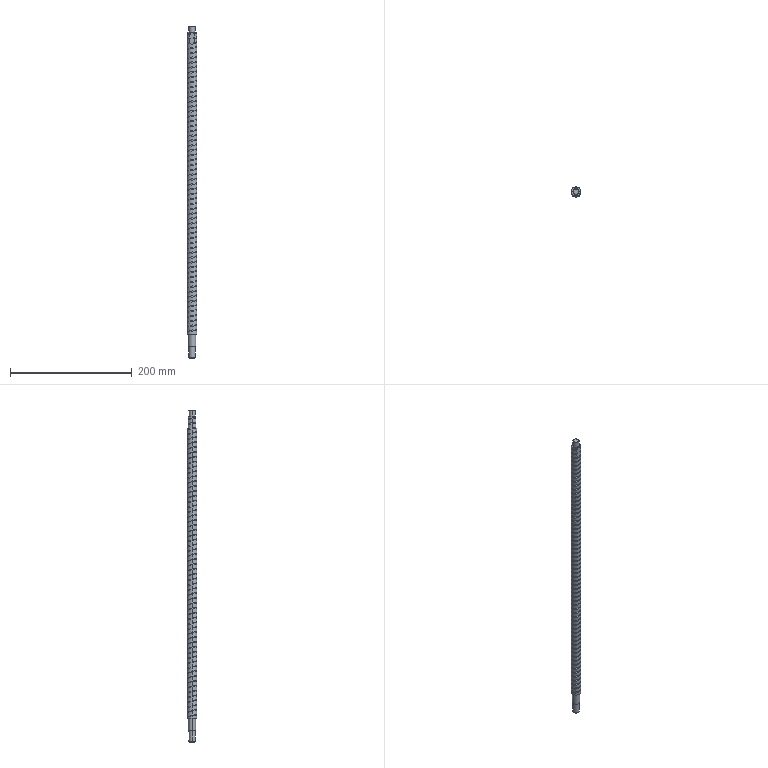Part | STEP file | Ball screw assembly SFUR1604-545 | 1 solid | 161 faces | box 16 x 16 x 545 mm | volume 99221 mm3 | cylinder 139 | plane 12 | spline 6 | cone 4 | commonest cylinder face diameters 16 x129 3 x4 10 x4 12 x2